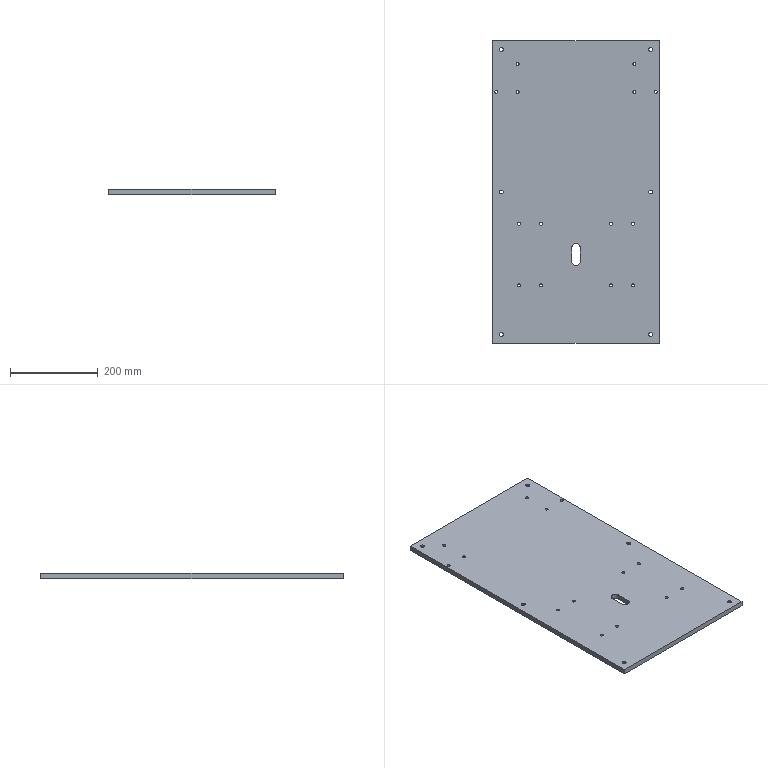Part | STEP file | X77-03004 | 1 solid | 70 faces | box 380 x 690 x 12 mm | volume 3118641 mm3 | cylinder 56 | plane 14 | commonest cylinder face diameters 6.8 x28 9 x12 15 x12 20 x4